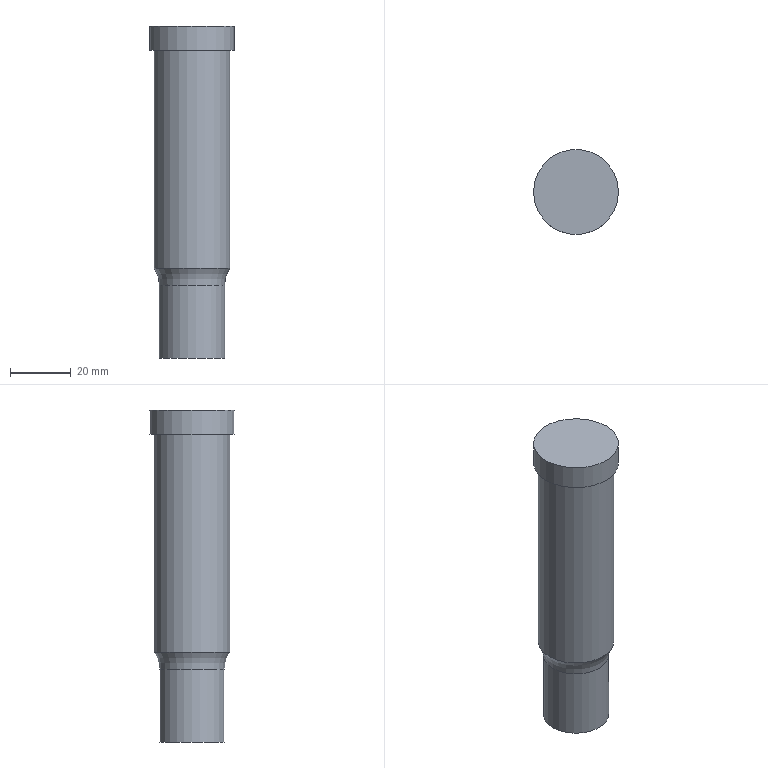Part | NX | features solid 2 | 1 solid | 7 faces | box 28 x 28 x 109.4 mm | volume 51146 mm3 | cylinder 3 | plane 3 | torus 1 | commonest cylinder face diameters 21.5 x1 25 x1 28 x1
STEP:
#1=CARTESIAN_POINT('',(1098.829,141.904,-7.483));
#2=VERTEX_POINT('',#1);
#3=CARTESIAN_POINT('',(1088.079,141.904,-7.483));
#4=DIRECTION('',(0.,0.,1.));
#5=DIRECTION('',(1.,0.,0.));
#6=AXIS2_PLACEMENT_3D('',#3,#4,#5);
#7=CIRCLE('',#6,10.75);
#8=EDGE_CURVE('',#2,#2,#7,.F.);
#9=ORIENTED_EDGE('',*,*,#8,.T.);
#10=EDGE_LOOP('',(#9));
#11=FACE_BOUND('',#10,.T.);
#12=CARTESIAN_POINT('',(1098.829,141.904,-31.4));
#13=VERTEX_POINT('',#12);
#14=CARTESIAN_POINT('',(1088.079,141.904,-31.4));
#15=DIRECTION('',(0.,0.,1.));
#16=DIRECTION('',(1.,0.,0.));
#17=AXIS2_PLACEMENT_3D('',#14,#15,#16);
#18=CIRCLE('',#17,10.75);
#19=EDGE_CURVE('',#13,#13,#18,.T.);
#20=ORIENTED_EDGE('',*,*,#19,.T.);
#21=EDGE_LOOP('',(#20));
#22=FACE_BOUND('',#21,.T.);
#23=CARTESIAN_POINT('',(1088.079,141.904,-21.632));
#24=DIRECTION('',(0.,0.,1.));
#25=DIRECTION('',(1.,0.,0.));
#26=AXIS2_PLACEMENT_3D('',#23,#24,#25);
#27=CYLINDRICAL_SURFACE('',#26,10.75);
#28=ADVANCED_FACE('',(#11,#22),#27,.T.);
#29=ORIENTED_EDGE('',*,*,#19,.F.);
#30=EDGE_LOOP('',(#29));
#31=FACE_BOUND('',#30,.T.);
#32=CARTESIAN_POINT('',(79.557,1232.968,-31.4));
#33=DIRECTION('',(0.,0.,1.));
#34=DIRECTION('',(-0.2588,-0.9659,0.));
#35=AXIS2_PLACEMENT_3D('',#32,#33,#34);
#36=PLANE('',#35);
#37=ADVANCED_FACE('',(#31),#36,.F.);
#38=CARTESIAN_POINT('',(1075.579,141.904,70.));
#39=VERTEX_POINT('',#38);
#40=CARTESIAN_POINT('',(1088.079,141.904,70.));
#41=DIRECTION('',(0.,0.,-1.));
#42=DIRECTION('',(-1.,0.,0.));
#43=AXIS2_PLACEMENT_3D('',#40,#41,#42);
#44=CIRCLE('',#43,12.5);
#45=EDGE_CURVE('',#39,#39,#44,.F.);
#46=ORIENTED_EDGE('',*,*,#45,.F.);
#47=EDGE_LOOP('',(#46));
#48=FACE_BOUND('',#47,.T.);
#49=CARTESIAN_POINT('',(1075.579,141.904,-1.832));
#50=VERTEX_POINT('',#49);
#51=CARTESIAN_POINT('',(1088.079,141.904,-1.832));
#52=DIRECTION('',(0.,0.,-1.));
#53=DIRECTION('',(-1.,0.,0.));
#54=AXIS2_PLACEMENT_3D('',#51,#52,#53);
#55=CIRCLE('',#54,12.5);
#56=EDGE_CURVE('',#50,#50,#55,.T.);
#57=ORIENTED_EDGE('',*,*,#56,.F.);
#58=EDGE_LOOP('',(#57));
#59=FACE_BOUND('',#58,.T.);
#60=CARTESIAN_POINT('',(1088.079,141.904,77.7));
#61=DIRECTION('',(0.,0.,-1.));
#62=DIRECTION('',(-1.,0.,0.));
#63=AXIS2_PLACEMENT_3D('',#60,#61,#62);
#64=CYLINDRICAL_SURFACE('',#63,12.5);
#65=ADVANCED_FACE('',(#48,#59),#64,.T.);
#66=ORIENTED_EDGE('',*,*,#8,.F.);
#67=EDGE_LOOP('',(#66));
#68=FACE_BOUND('',#67,.T.);
#69=ORIENTED_EDGE('',*,*,#56,.T.);
#70=EDGE_LOOP('',(#69));
#71=FACE_BOUND('',#70,.T.);
#72=CARTESIAN_POINT('',(1088.079,141.904,-7.483));
#73=DIRECTION('',(0.,0.,1.));
#74=DIRECTION('',(1.,0.,0.));
#75=AXIS2_PLACEMENT_3D('',#72,#73,#74);
#76=TOROIDAL_SURFACE('',#75,20.75,10.);
#77=ADVANCED_FACE('',(#68,#71),#76,.F.);
#78=CARTESIAN_POINT('',(1074.079,141.904,78.));
#79=VERTEX_POINT('',#78);
#80=CARTESIAN_POINT('',(1088.079,141.904,78.));
#81=DIRECTION('',(0.,0.,-1.));
#82=DIRECTION('',(-1.,0.,0.));
#83=AXIS2_PLACEMENT_3D('',#80,#81,#82);
#84=CIRCLE('',#83,14.);
#85=EDGE_CURVE('',#79,#79,#84,.T.);
#86=ORIENTED_EDGE('',*,*,#85,.T.);
#87=EDGE_LOOP('',(#86));
#88=FACE_BOUND('',#87,.T.);
#89=CARTESIAN_POINT('',(1074.079,141.904,70.));
#90=VERTEX_POINT('',#89);
#91=CARTESIAN_POINT('',(1088.079,141.904,70.));
#92=DIRECTION('',(0.,0.,-1.));
#93=DIRECTION('',(-1.,0.,0.));
#94=AXIS2_PLACEMENT_3D('',#91,#92,#93);
#95=CIRCLE('',#94,14.);
#96=EDGE_CURVE('',#90,#90,#95,.T.);
#97=ORIENTED_EDGE('',*,*,#96,.F.);
#98=EDGE_LOOP('',(#97));
#99=FACE_BOUND('',#98,.T.);
#100=CARTESIAN_POINT('',(1088.079,141.904,77.7));
#101=DIRECTION('',(0.,0.,-1.));
#102=DIRECTION('',(-1.,0.,0.));
#103=AXIS2_PLACEMENT_3D('',#100,#101,#102);
#104=CYLINDRICAL_SURFACE('',#103,14.);
#105=ADVANCED_FACE('',(#88,#99),#104,.T.);
#106=ORIENTED_EDGE('',*,*,#45,.T.);
#107=EDGE_LOOP('',(#106));
#108=FACE_BOUND('',#107,.T.);
#109=ORIENTED_EDGE('',*,*,#96,.T.);
#110=EDGE_LOOP('',(#109));
#111=FACE_BOUND('',#110,.T.);
#112=CARTESIAN_POINT('',(1088.079,141.904,70.));
#113=DIRECTION('',(0.,0.,-1.));
#114=DIRECTION('',(-1.,0.,0.));
#115=AXIS2_PLACEMENT_3D('',#112,#113,#114);
#116=PLANE('',#115);
#117=ADVANCED_FACE('',(#108,#111),#116,.T.);
#118=ORIENTED_EDGE('',*,*,#85,.F.);
#119=EDGE_LOOP('',(#118));
#120=FACE_BOUND('',#119,.T.);
#121=CARTESIAN_POINT('',(1889.158,0.000000688,78.));
#122=DIRECTION('',(0.,0.,-1.));
#123=DIRECTION('',(1.,0.,0.));
#124=AXIS2_PLACEMENT_3D('',#121,#122,#123);
#125=PLANE('',#124);
#126=ADVANCED_FACE('',(#120),#125,.F.);
#127=CLOSED_SHELL('',(#28,#37,#65,#77,#105,#117,#126));
#128=MANIFOLD_SOLID_BREP('',#127);
#129=(LENGTH_UNIT()NAMED_UNIT(*)SI_UNIT(.MILLI.,.METRE.));
#130=UNCERTAINTY_MEASURE_WITH_UNIT(LENGTH_MEASURE(0.00001),#129,'','');
#131=(NAMED_UNIT(*)PLANE_ANGLE_UNIT()SI_UNIT($,.RADIAN.));
#132=(NAMED_UNIT(*)SI_UNIT($,.STERADIAN.)SOLID_ANGLE_UNIT());
#133=(GEOMETRIC_REPRESENTATION_CONTEXT(3)GLOBAL_UNCERTAINTY_ASSIGNED_CONTEXT((#130))GLOBAL_UNIT_ASSIGNED_CONTEXT((#129,#131,#132))REPRESENTATION_CONTEXT('',''));
#134=ADVANCED_BREP_SHAPE_REPRESENTATION('',(#128),#133);